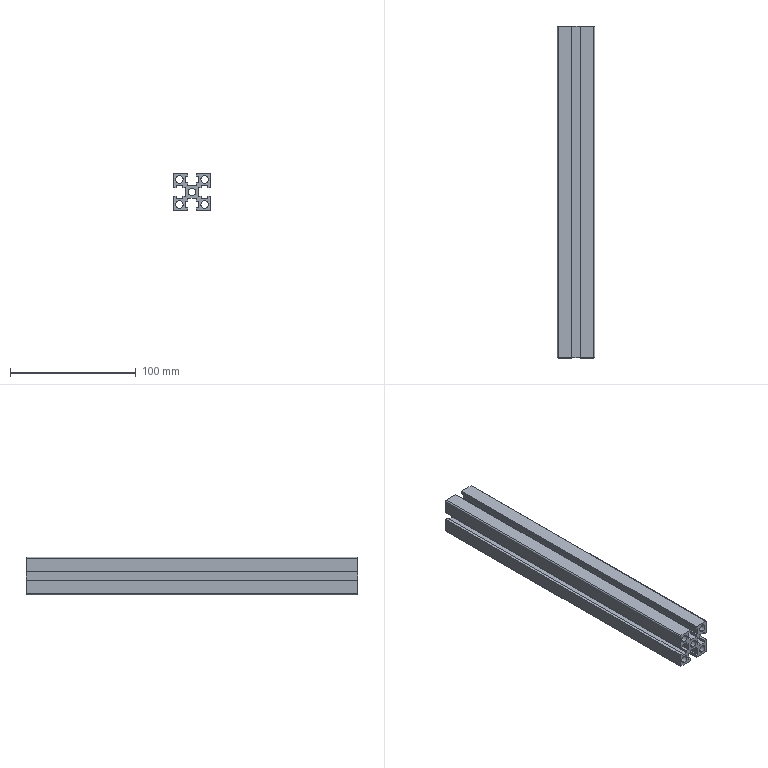Part | STEP file | 02-15 Belt line connecting rod | 1 solid | 68 faces | box 30 x 264 x 30 mm | volume 111601 mm3 | plane 54 | cylinder 14 | commonest cylinder face diameters 6 x10 2 x4